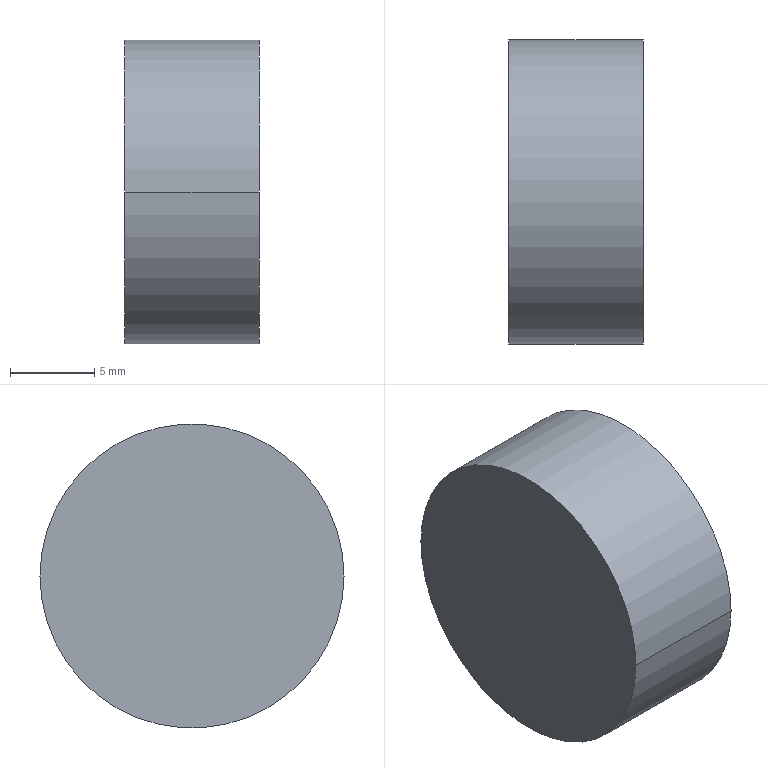Part | STEP file | _X2_7FC5724752A070ED7BA1_X0_1_9 | 1 solid | 4 faces | box 8 x 18.069 x 18.069 mm | volume 2051 mm3 | plane 2 | cylinder 2 | commonest cylinder face diameters 18.069 x2
STEP:
#1=CARTESIAN_POINT('',(0.,0.,0.));
#2=DIRECTION('',(0.,0.,1.));
#3=DIRECTION('',(1.,0.,0.));
#4=AXIS2_PLACEMENT_3D('',#1,#2,#3);
#5=CARTESIAN_POINT('',(-37.,9.035,0.));
#6=VERTEX_POINT('',#5);
#7=CARTESIAN_POINT('',(-37.,-9.035,0.));
#8=VERTEX_POINT('',#7);
#9=CARTESIAN_POINT('',(-37.,0.,0.));
#10=DIRECTION('',(-1.,0.,0.));
#11=DIRECTION('',(0.,1.,0.));
#12=AXIS2_PLACEMENT_3D('',#9,#10,#11);
#13=CIRCLE('',#12,9.035);
#14=CARTESIAN_POINT('',(-37.,0.,0.));
#15=DIRECTION('',(-1.,0.,0.));
#16=DIRECTION('',(0.,-1.,0.));
#17=AXIS2_PLACEMENT_3D('',#14,#15,#16);
#18=PLANE('',#17);
#19=CARTESIAN_POINT('',(0.,0.));
#20=DIRECTION('',(-1.,0.));
#21=AXIS2_PLACEMENT_2D('',#19,#20);
#22=CIRCLE('',#21,9.035);
#23=(GEOMETRIC_REPRESENTATION_CONTEXT(2)PARAMETRIC_REPRESENTATION_CONTEXT()REPRESENTATION_CONTEXT('',''));
#24=DEFINITIONAL_REPRESENTATION('',(#22),#23);
#25=PCURVE('',#18,#24);
#26=CARTESIAN_POINT('',(-37.,0.,0.));
#27=DIRECTION('',(1.,0.,0.));
#28=DIRECTION('',(0.,1.,0.));
#29=AXIS2_PLACEMENT_3D('',#26,#27,#28);
#30=CYLINDRICAL_SURFACE('',#29,9.035);
#31=CARTESIAN_POINT('',(6.283,0.));
#32=DIRECTION('',(-1.,0.));
#33=VECTOR('',#32,1.);
#34=LINE('',#31,#33);
#35=(GEOMETRIC_REPRESENTATION_CONTEXT(2)PARAMETRIC_REPRESENTATION_CONTEXT()REPRESENTATION_CONTEXT('',''));
#36=DEFINITIONAL_REPRESENTATION('',(#34),#35);
#37=PCURVE('',#30,#36);
#38=SURFACE_CURVE('',#13,(#25,#37),.PCURVE_S1.);
#39=EDGE_CURVE('',#6,#8,#38,.T.);
#40=ORIENTED_EDGE('',*,*,#39,.F.);
#41=CARTESIAN_POINT('',(-37.,0.,0.));
#42=DIRECTION('',(-1.,0.,0.));
#43=DIRECTION('',(0.,-1.,0.));
#44=AXIS2_PLACEMENT_3D('',#41,#42,#43);
#45=CIRCLE('',#44,9.035);
#46=CARTESIAN_POINT('',(0.,0.));
#47=DIRECTION('',(1.,0.));
#48=AXIS2_PLACEMENT_2D('',#46,#47);
#49=CIRCLE('',#48,9.035);
#50=(GEOMETRIC_REPRESENTATION_CONTEXT(2)PARAMETRIC_REPRESENTATION_CONTEXT()REPRESENTATION_CONTEXT('',''));
#51=DEFINITIONAL_REPRESENTATION('',(#49),#50);
#52=PCURVE('',#18,#51);
#53=CARTESIAN_POINT('',(-37.,0.,0.));
#54=DIRECTION('',(1.,0.,0.));
#55=DIRECTION('',(0.,1.,0.));
#56=AXIS2_PLACEMENT_3D('',#53,#54,#55);
#57=CYLINDRICAL_SURFACE('',#56,9.035);
#58=CARTESIAN_POINT('',(3.142,0.));
#59=DIRECTION('',(-1.,0.));
#60=VECTOR('',#59,1.);
#61=LINE('',#58,#60);
#62=(GEOMETRIC_REPRESENTATION_CONTEXT(2)PARAMETRIC_REPRESENTATION_CONTEXT()REPRESENTATION_CONTEXT('',''));
#63=DEFINITIONAL_REPRESENTATION('',(#61),#62);
#64=PCURVE('',#57,#63);
#65=SURFACE_CURVE('',#45,(#52,#64),.PCURVE_S1.);
#66=EDGE_CURVE('',#8,#6,#65,.T.);
#67=ORIENTED_EDGE('',*,*,#66,.F.);
#68=EDGE_LOOP('',(#40,#67));
#69=FACE_BOUND('',#68,.F.);
#70=ADVANCED_FACE('',(#69),#18,.T.);
#71=CARTESIAN_POINT('',(-29.,9.035,0.));
#72=VERTEX_POINT('',#71);
#73=CARTESIAN_POINT('',(-37.,9.035,0.));
#74=DIRECTION('',(1.,0.,0.));
#75=VECTOR('',#74,1.);
#76=LINE('',#73,#75);
#77=CARTESIAN_POINT('',(6.283,0.));
#78=DIRECTION('',(0.,1.));
#79=VECTOR('',#78,1.);
#80=LINE('',#77,#79);
#81=(GEOMETRIC_REPRESENTATION_CONTEXT(2)PARAMETRIC_REPRESENTATION_CONTEXT()REPRESENTATION_CONTEXT('',''));
#82=DEFINITIONAL_REPRESENTATION('',(#80),#81);
#83=PCURVE('',#30,#82);
#84=CARTESIAN_POINT('',(0.,0.));
#85=DIRECTION('',(0.,1.));
#86=VECTOR('',#85,1.);
#87=LINE('',#84,#86);
#88=(GEOMETRIC_REPRESENTATION_CONTEXT(2)PARAMETRIC_REPRESENTATION_CONTEXT()REPRESENTATION_CONTEXT('',''));
#89=DEFINITIONAL_REPRESENTATION('',(#87),#88);
#90=PCURVE('',#57,#89);
#91=SURFACE_CURVE('',#76,(#83,#90),.PCURVE_S1.);
#92=EDGE_CURVE('',#6,#72,#91,.T.);
#93=ORIENTED_EDGE('',*,*,#92,.T.);
#94=CARTESIAN_POINT('',(-29.,-9.035,0.));
#95=VERTEX_POINT('',#94);
#96=CARTESIAN_POINT('',(-29.,0.,0.));
#97=DIRECTION('',(1.,0.,0.));
#98=DIRECTION('',(0.,-1.,0.));
#99=AXIS2_PLACEMENT_3D('',#96,#97,#98);
#100=CIRCLE('',#99,9.035);
#101=CARTESIAN_POINT('',(3.142,8.));
#102=DIRECTION('',(1.,0.));
#103=VECTOR('',#102,1.);
#104=LINE('',#101,#103);
#105=(GEOMETRIC_REPRESENTATION_CONTEXT(2)PARAMETRIC_REPRESENTATION_CONTEXT()REPRESENTATION_CONTEXT('',''));
#106=DEFINITIONAL_REPRESENTATION('',(#104),#105);
#107=PCURVE('',#30,#106);
#108=CARTESIAN_POINT('',(-29.,0.,0.));
#109=DIRECTION('',(-1.,0.,0.));
#110=DIRECTION('',(0.,-1.,0.));
#111=AXIS2_PLACEMENT_3D('',#108,#109,#110);
#112=PLANE('',#111);
#113=CARTESIAN_POINT('',(9.035,0.));
#114=CARTESIAN_POINT('',(9.035,-15.649));
#115=CARTESIAN_POINT('',(-4.517,-7.824));
#116=CARTESIAN_POINT('',(-18.069,0.));
#117=CARTESIAN_POINT('',(-4.517,7.824));
#118=CARTESIAN_POINT('',(9.035,15.649));
#119=CARTESIAN_POINT('',(9.035,0.));
#120=(BOUNDED_CURVE()B_SPLINE_CURVE(2,(#113,#114,#115,#116,#117,#118,#119),.UNSPECIFIED.,.T.,.F.)B_SPLINE_CURVE_WITH_KNOTS((1,2,2,2,2,1),(-2.094,0.,2.094,4.189,6.283,8.378),.UNSPECIFIED.)CURVE()GEOMETRIC_REPRESENTATION_ITEM()RATIONAL_B_SPLINE_CURVE((1.,0.5,1.,0.5,1.,0.5,1.))REPRESENTATION_ITEM(''));
#121=(GEOMETRIC_REPRESENTATION_CONTEXT(2)PARAMETRIC_REPRESENTATION_CONTEXT()REPRESENTATION_CONTEXT('',''));
#122=DEFINITIONAL_REPRESENTATION('',(#120),#121);
#123=PCURVE('',#112,#122);
#124=SURFACE_CURVE('',#100,(#107,#123),.PCURVE_S1.);
#125=EDGE_CURVE('',#95,#72,#124,.T.);
#126=ORIENTED_EDGE('',*,*,#125,.F.);
#127=CARTESIAN_POINT('',(-37.,-9.035,0.));
#128=DIRECTION('',(1.,0.,0.));
#129=VECTOR('',#128,1.);
#130=LINE('',#127,#129);
#131=CARTESIAN_POINT('',(3.142,0.));
#132=DIRECTION('',(0.,1.));
#133=VECTOR('',#132,1.);
#134=LINE('',#131,#133);
#135=(GEOMETRIC_REPRESENTATION_CONTEXT(2)PARAMETRIC_REPRESENTATION_CONTEXT()REPRESENTATION_CONTEXT('',''));
#136=DEFINITIONAL_REPRESENTATION('',(#134),#135);
#137=PCURVE('',#30,#136);
#138=CARTESIAN_POINT('',(3.142,0.));
#139=DIRECTION('',(0.,1.));
#140=VECTOR('',#139,1.);
#141=LINE('',#138,#140);
#142=(GEOMETRIC_REPRESENTATION_CONTEXT(2)PARAMETRIC_REPRESENTATION_CONTEXT()REPRESENTATION_CONTEXT('',''));
#143=DEFINITIONAL_REPRESENTATION('',(#141),#142);
#144=PCURVE('',#57,#143);
#145=SURFACE_CURVE('',#130,(#137,#144),.PCURVE_S1.);
#146=EDGE_CURVE('',#8,#95,#145,.T.);
#147=ORIENTED_EDGE('',*,*,#146,.F.);
#148=ORIENTED_EDGE('',*,*,#39,.F.);
#149=EDGE_LOOP('',(#93,#126,#147,#148));
#150=FACE_BOUND('',#149,.T.);
#151=ADVANCED_FACE('',(#150),#30,.T.);
#152=ORIENTED_EDGE('',*,*,#146,.T.);
#153=CARTESIAN_POINT('',(-29.,0.,0.));
#154=DIRECTION('',(1.,0.,0.));
#155=DIRECTION('',(0.,1.,0.));
#156=AXIS2_PLACEMENT_3D('',#153,#154,#155);
#157=CIRCLE('',#156,9.035);
#158=CARTESIAN_POINT('',(0.,8.));
#159=DIRECTION('',(1.,0.));
#160=VECTOR('',#159,1.);
#161=LINE('',#158,#160);
#162=(GEOMETRIC_REPRESENTATION_CONTEXT(2)PARAMETRIC_REPRESENTATION_CONTEXT()REPRESENTATION_CONTEXT('',''));
#163=DEFINITIONAL_REPRESENTATION('',(#161),#162);
#164=PCURVE('',#57,#163);
#165=CARTESIAN_POINT('',(-9.035,0.));
#166=CARTESIAN_POINT('',(-9.035,15.649));
#167=CARTESIAN_POINT('',(4.517,7.824));
#168=CARTESIAN_POINT('',(18.069,0.));
#169=CARTESIAN_POINT('',(4.517,-7.824));
#170=CARTESIAN_POINT('',(-9.035,-15.649));
#171=CARTESIAN_POINT('',(-9.035,0.));
#172=(BOUNDED_CURVE()B_SPLINE_CURVE(2,(#165,#166,#167,#168,#169,#170,#171),.UNSPECIFIED.,.T.,.F.)B_SPLINE_CURVE_WITH_KNOTS((1,2,2,2,2,1),(-2.094,0.,2.094,4.189,6.283,8.378),.UNSPECIFIED.)CURVE()GEOMETRIC_REPRESENTATION_ITEM()RATIONAL_B_SPLINE_CURVE((1.,0.5,1.,0.5,1.,0.5,1.))REPRESENTATION_ITEM(''));
#173=(GEOMETRIC_REPRESENTATION_CONTEXT(2)PARAMETRIC_REPRESENTATION_CONTEXT()REPRESENTATION_CONTEXT('',''));
#174=DEFINITIONAL_REPRESENTATION('',(#172),#173);
#175=PCURVE('',#112,#174);
#176=SURFACE_CURVE('',#157,(#164,#175),.PCURVE_S1.);
#177=EDGE_CURVE('',#72,#95,#176,.T.);
#178=ORIENTED_EDGE('',*,*,#177,.F.);
#179=ORIENTED_EDGE('',*,*,#92,.F.);
#180=ORIENTED_EDGE('',*,*,#66,.F.);
#181=EDGE_LOOP('',(#152,#178,#179,#180));
#182=FACE_BOUND('',#181,.T.);
#183=ADVANCED_FACE('',(#182),#57,.T.);
#184=ORIENTED_EDGE('',*,*,#125,.F.);
#185=ORIENTED_EDGE('',*,*,#177,.F.);
#186=EDGE_LOOP('',(#184,#185));
#187=FACE_BOUND('',#186,.F.);
#188=ADVANCED_FACE('',(#187),#112,.F.);
#189=CLOSED_SHELL('',(#70,#151,#183,#188));
#190=MANIFOLD_SOLID_BREP('',#189);
#191=(LENGTH_UNIT()NAMED_UNIT(*)SI_UNIT(.MILLI.,.METRE.));
#192=UNCERTAINTY_MEASURE_WITH_UNIT(LENGTH_MEASURE(0.0000001),#191,'','');
#193=(NAMED_UNIT(*)PLANE_ANGLE_UNIT()SI_UNIT($,.RADIAN.));
#194=(NAMED_UNIT(*)SI_UNIT($,.STERADIAN.)SOLID_ANGLE_UNIT());
#195=(GEOMETRIC_REPRESENTATION_CONTEXT(3)GLOBAL_UNCERTAINTY_ASSIGNED_CONTEXT((#192))GLOBAL_UNIT_ASSIGNED_CONTEXT((#191,#193,#194))REPRESENTATION_CONTEXT('',''));
#196=ADVANCED_BREP_SHAPE_REPRESENTATION('',(#4,#190),#195);